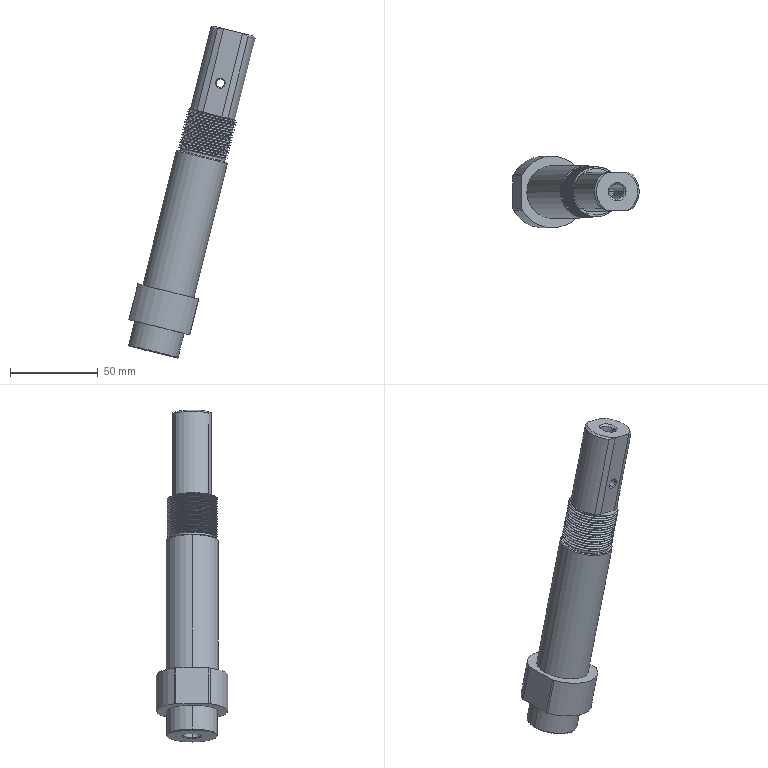Part | SolidWorks | features BaseBody 1 | 1 solid | 121 faces | box 72.158 x 40.8 x 189.343 mm | volume 126337 mm3 | cylinder 84 | cone 17 | plane 16 | spline 4 | commonest cylinder face diameters 26.5 x33 28.6 x32 4 x4 40.8 x3 4.8 x2 8.5 x2